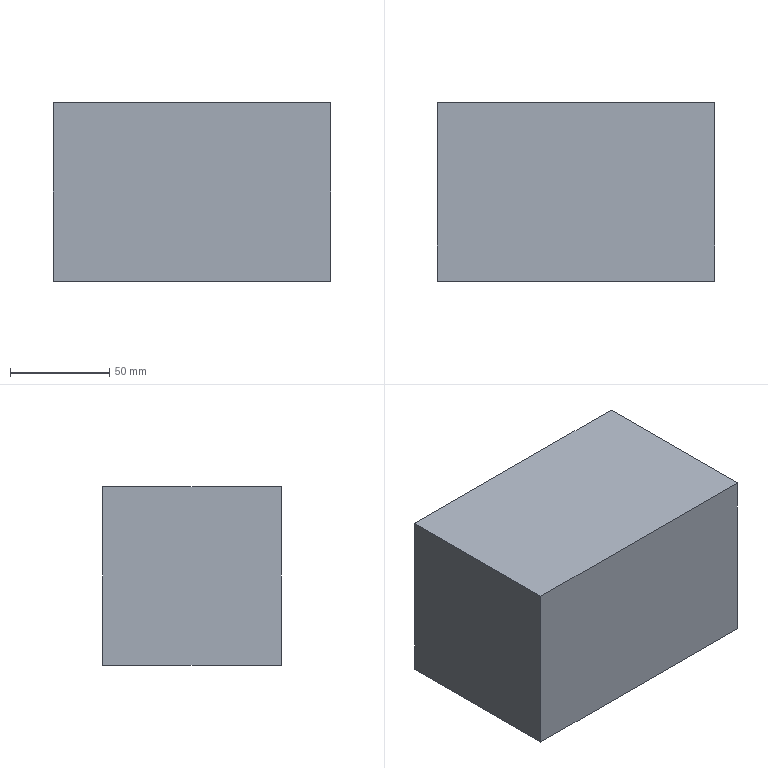Part | SolidWorks | features Extrusion 1 | 1 solid | 6 faces | box 140 x 90 x 90 mm | volume 1134000 mm3 | plane 6
STEP:
#1=CARTESIAN_POINT('',(-70.,45.,45.));
#2=VERTEX_POINT('',#1);
#3=CARTESIAN_POINT('',(-70.,-45.,45.));
#4=VERTEX_POINT('',#3);
#5=CARTESIAN_POINT('',(-70.,45.,45.));
#6=DIRECTION('',(0.,-1.,0.));
#7=VECTOR('',#6,1000.);
#8=LINE('',#5,#7);
#9=EDGE_CURVE('',#2,#4,#8,.T.);
#10=ORIENTED_EDGE('',*,*,#9,.F.);
#11=CARTESIAN_POINT('',(-70.,45.,-45.));
#12=VERTEX_POINT('',#11);
#13=CARTESIAN_POINT('',(-70.,45.,-45.));
#14=DIRECTION('',(0.,0.,1.));
#15=VECTOR('',#14,1000.);
#16=LINE('',#13,#15);
#17=EDGE_CURVE('',#12,#2,#16,.T.);
#18=ORIENTED_EDGE('',*,*,#17,.F.);
#19=CARTESIAN_POINT('',(-70.,-45.,-45.));
#20=VERTEX_POINT('',#19);
#21=CARTESIAN_POINT('',(-70.,45.,-45.));
#22=DIRECTION('',(0.,-1.,0.));
#23=VECTOR('',#22,1000.);
#24=LINE('',#21,#23);
#25=EDGE_CURVE('',#12,#20,#24,.T.);
#26=ORIENTED_EDGE('',*,*,#25,.T.);
#27=CARTESIAN_POINT('',(-70.,-45.,-45.));
#28=DIRECTION('',(0.,0.,1.));
#29=VECTOR('',#28,1000.);
#30=LINE('',#27,#29);
#31=EDGE_CURVE('',#20,#4,#30,.T.);
#32=ORIENTED_EDGE('',*,*,#31,.T.);
#33=EDGE_LOOP('',(#10,#18,#26,#32));
#34=FACE_OUTER_BOUND('',#33,.T.);
#35=CARTESIAN_POINT('',(-70.,45.,-45.));
#36=DIRECTION('',(-1.,0.,0.));
#37=DIRECTION('',(0.,0.,1.));
#38=AXIS2_PLACEMENT_3D('',#35,#36,#37);
#39=PLANE('',#38);
#40=ADVANCED_FACE('',(#34),#39,.T.);
#41=CARTESIAN_POINT('',(70.,45.,45.));
#42=VERTEX_POINT('',#41);
#43=CARTESIAN_POINT('',(70.,45.,45.));
#44=DIRECTION('',(-1.,0.,0.));
#45=VECTOR('',#44,1000.);
#46=LINE('',#43,#45);
#47=EDGE_CURVE('',#42,#2,#46,.T.);
#48=ORIENTED_EDGE('',*,*,#47,.F.);
#49=CARTESIAN_POINT('',(70.,45.,-45.));
#50=VERTEX_POINT('',#49);
#51=CARTESIAN_POINT('',(70.,45.,-45.));
#52=DIRECTION('',(0.,0.,1.));
#53=VECTOR('',#52,1000.);
#54=LINE('',#51,#53);
#55=EDGE_CURVE('',#50,#42,#54,.T.);
#56=ORIENTED_EDGE('',*,*,#55,.F.);
#57=CARTESIAN_POINT('',(70.,45.,-45.));
#58=DIRECTION('',(-1.,0.,0.));
#59=VECTOR('',#58,1000.);
#60=LINE('',#57,#59);
#61=EDGE_CURVE('',#50,#12,#60,.T.);
#62=ORIENTED_EDGE('',*,*,#61,.T.);
#63=ORIENTED_EDGE('',*,*,#17,.T.);
#64=EDGE_LOOP('',(#48,#56,#62,#63));
#65=FACE_OUTER_BOUND('',#64,.T.);
#66=CARTESIAN_POINT('',(70.,45.,-45.));
#67=DIRECTION('',(0.,1.,0.));
#68=DIRECTION('',(0.,0.,1.));
#69=AXIS2_PLACEMENT_3D('',#66,#67,#68);
#70=PLANE('',#69);
#71=ADVANCED_FACE('',(#65),#70,.T.);
#72=CARTESIAN_POINT('',(70.,-45.,45.));
#73=VERTEX_POINT('',#72);
#74=CARTESIAN_POINT('',(70.,-45.,45.));
#75=DIRECTION('',(0.,1.,0.));
#76=VECTOR('',#75,1000.);
#77=LINE('',#74,#76);
#78=EDGE_CURVE('',#73,#42,#77,.T.);
#79=ORIENTED_EDGE('',*,*,#78,.F.);
#80=CARTESIAN_POINT('',(70.,-45.,-45.));
#81=VERTEX_POINT('',#80);
#82=CARTESIAN_POINT('',(70.,-45.,-45.));
#83=DIRECTION('',(0.,0.,1.));
#84=VECTOR('',#83,1000.);
#85=LINE('',#82,#84);
#86=EDGE_CURVE('',#81,#73,#85,.T.);
#87=ORIENTED_EDGE('',*,*,#86,.F.);
#88=CARTESIAN_POINT('',(70.,-45.,-45.));
#89=DIRECTION('',(0.,1.,0.));
#90=VECTOR('',#89,1000.);
#91=LINE('',#88,#90);
#92=EDGE_CURVE('',#81,#50,#91,.T.);
#93=ORIENTED_EDGE('',*,*,#92,.T.);
#94=ORIENTED_EDGE('',*,*,#55,.T.);
#95=EDGE_LOOP('',(#79,#87,#93,#94));
#96=FACE_OUTER_BOUND('',#95,.T.);
#97=CARTESIAN_POINT('',(70.,-45.,-45.));
#98=DIRECTION('',(1.,0.,0.));
#99=DIRECTION('',(0.,0.,-1.));
#100=AXIS2_PLACEMENT_3D('',#97,#98,#99);
#101=PLANE('',#100);
#102=ADVANCED_FACE('',(#96),#101,.T.);
#103=CARTESIAN_POINT('',(-70.,-45.,45.));
#104=DIRECTION('',(1.,0.,0.));
#105=VECTOR('',#104,1000.);
#106=LINE('',#103,#105);
#107=EDGE_CURVE('',#4,#73,#106,.T.);
#108=ORIENTED_EDGE('',*,*,#107,.F.);
#109=ORIENTED_EDGE('',*,*,#31,.F.);
#110=CARTESIAN_POINT('',(-70.,-45.,-45.));
#111=DIRECTION('',(1.,0.,0.));
#112=VECTOR('',#111,1000.);
#113=LINE('',#110,#112);
#114=EDGE_CURVE('',#20,#81,#113,.T.);
#115=ORIENTED_EDGE('',*,*,#114,.T.);
#116=ORIENTED_EDGE('',*,*,#86,.T.);
#117=EDGE_LOOP('',(#108,#109,#115,#116));
#118=FACE_OUTER_BOUND('',#117,.T.);
#119=CARTESIAN_POINT('',(-70.,-45.,-45.));
#120=DIRECTION('',(0.,-1.,0.));
#121=DIRECTION('',(0.,0.,-1.));
#122=AXIS2_PLACEMENT_3D('',#119,#120,#121);
#123=PLANE('',#122);
#124=ADVANCED_FACE('',(#118),#123,.T.);
#125=ORIENTED_EDGE('',*,*,#25,.F.);
#126=ORIENTED_EDGE('',*,*,#61,.F.);
#127=ORIENTED_EDGE('',*,*,#92,.F.);
#128=ORIENTED_EDGE('',*,*,#114,.F.);
#129=EDGE_LOOP('',(#125,#126,#127,#128));
#130=FACE_OUTER_BOUND('',#129,.T.);
#131=CARTESIAN_POINT('',(0.,0.,-45.));
#132=DIRECTION('',(0.,0.,1.));
#133=DIRECTION('',(1.,0.,0.));
#134=AXIS2_PLACEMENT_3D('',#131,#132,#133);
#135=PLANE('',#134);
#136=ADVANCED_FACE('',(#130),#135,.F.);
#137=ORIENTED_EDGE('',*,*,#9,.T.);
#138=ORIENTED_EDGE('',*,*,#107,.T.);
#139=ORIENTED_EDGE('',*,*,#78,.T.);
#140=ORIENTED_EDGE('',*,*,#47,.T.);
#141=EDGE_LOOP('',(#137,#138,#139,#140));
#142=FACE_OUTER_BOUND('',#141,.T.);
#143=CARTESIAN_POINT('',(0.,0.,45.));
#144=DIRECTION('',(0.,0.,1.));
#145=DIRECTION('',(1.,0.,0.));
#146=AXIS2_PLACEMENT_3D('',#143,#144,#145);
#147=PLANE('',#146);
#148=ADVANCED_FACE('',(#142),#147,.T.);
#149=CLOSED_SHELL('',(#40,#71,#102,#124,#136,#148));
#150=MANIFOLD_SOLID_BREP('',#149);
#151=CARTESIAN_POINT('',(0.,0.,0.));
#152=DIRECTION('',(0.,0.,1.));
#153=DIRECTION('',(1.,0.,0.));
#154=AXIS2_PLACEMENT_3D('',#151,#152,#153);
#155=(LENGTH_UNIT()NAMED_UNIT(*)SI_UNIT(.MILLI.,.METRE.));
#156=UNCERTAINTY_MEASURE_WITH_UNIT(LENGTH_MEASURE(0.00001),#155,'','');
#157=(NAMED_UNIT(*)PLANE_ANGLE_UNIT()SI_UNIT($,.RADIAN.));
#158=(NAMED_UNIT(*)SI_UNIT($,.STERADIAN.)SOLID_ANGLE_UNIT());
#159=(GEOMETRIC_REPRESENTATION_CONTEXT(3)GLOBAL_UNCERTAINTY_ASSIGNED_CONTEXT((#156))GLOBAL_UNIT_ASSIGNED_CONTEXT((#155,#157,#158))REPRESENTATION_CONTEXT('',''));
#160=ADVANCED_BREP_SHAPE_REPRESENTATION('',(#150,#154),#159);